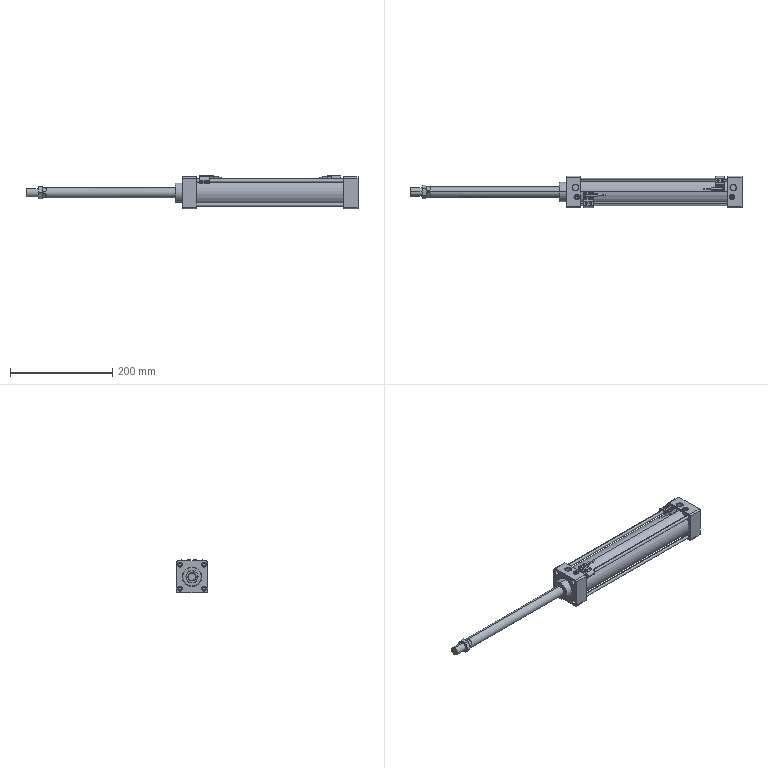Part | SolidWorks | 7 solids | 412 faces | box 650 x 62 x 64.972 mm | volume 512246 mm3 | plane 180 | cylinder 152 | cone 78 | torus 2 | commonest cylinder face diameters 6 x18 4.917 x16 9.5 x16 0.4 x8 0.8 x8 1 x8